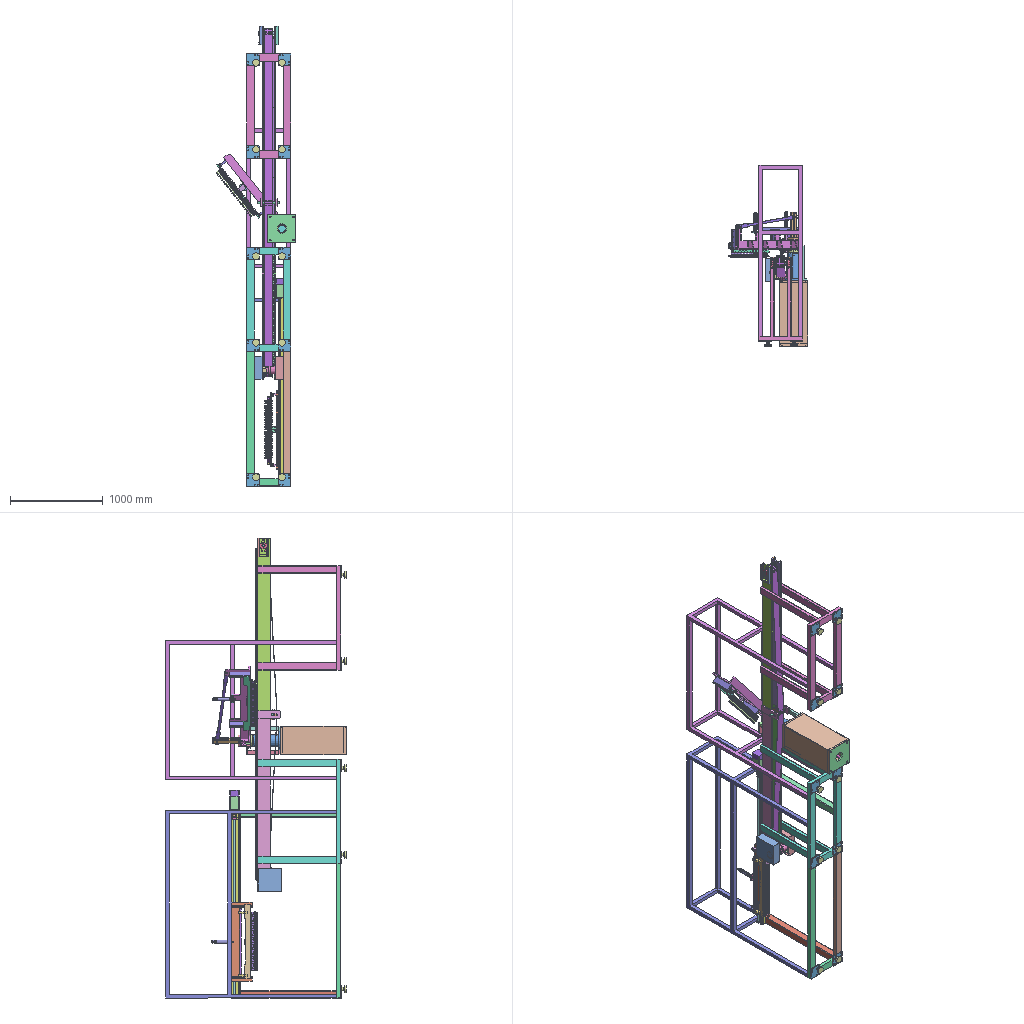Assembly | STEP file | 79 different items | 846 placed | box 859 x 1942 x 4946 mm
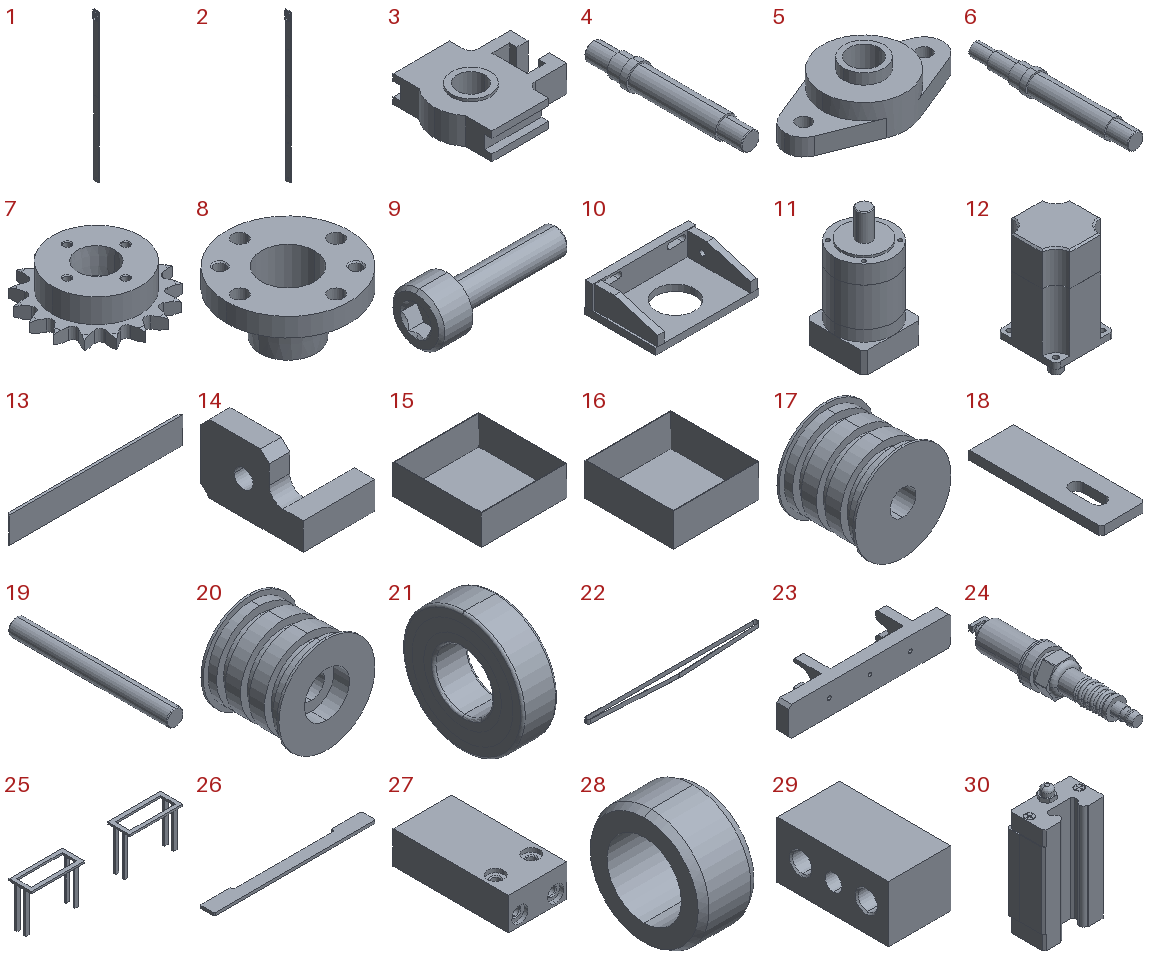Parts list (item | name | quantity | parent item | size | volume):
1 | 012-6-07-01-2 | x1 | in 12-06-07-00-2 | 51 x 134.1 x 3800 mm | 8306378 mm3
2 | 012-6-07-02-2 | x1 | in 12-06-07-00-2 | 51 x 134.1 x 3800 mm | 8297269 mm3
3 | UCT205 | x2 | in 12-06-07-00-2 | 94 x 89 x 34 mm | 126176 mm3
4 | 012-6-07-04 | x1 | in 12-06-07-00-2 | 35 x 216.4 x 35 mm | 140753 mm3
5 | UCFL205 | x2 | in 12-06-07-00-2 | 130 x 68 x 35.7 mm | 116034 mm3
6 | 012-6-07-05 | x1 | in 12-06-07-00-2 | 35 x 249.4 x 35 mm | 151867 mm3
7 | LFSP40B17_20_Asp | x2 | in LFSP40B17_20_A_LFSP40B17-20-A | 75.676 x 75.353 x 22 mm | 49189 mm3
8 | LFSP35B_20_boltbushing | x2 | in LFSP40B17_20_A_LFSP40B17-20-A | 46 x 46 x 23 mm | 9749 mm3
9 | LFSP35B20boltbolt | x8 | in LFSP40B17_20_A_LFSP40B17-20-A | 27 x 10 x 10 mm | 802.883 mm3
10 | 012-6-07-07 | x1 | in 12-06-07-00-2 | 160 x 110 x 46.5 mm | 267111 mm3
11 | PL80-40 | x2 | in 12-06-07-00-2, Reducer 2012-6-19 | 80 x 80 x 162 mm | 651730 mm3
12 | 1FL40-44-0AF21-0AA0 | x2 | in 12-06-07-00-2, Reducer 2012-6-19 | 80 x 80 x 173 mm | 725829 mm3
13 | 012-6-07-08 | x3 | in 12-06-07-00-2 | 750 x 12 x 114 mm | 828876 mm3
14 | 012-6-07-010 | x1 | in 12-06-07-00-2 | 42 x 60 x 40 mm | 27374 mm3
15 | 012-6-07-011 | x1 | in 12-06-07-00-2 | 247 x 253 x 86 mm | 291638 mm3
16 | 012-6-07-012 | x1 | in 12-06-07-00-2 | 247 x 253 x 95 mm | 309494 mm3
17 | 012-6-07-016 | x2 | in 12-06-07-00-2 | 111 x 90 x 111 mm | 582989 mm3
18 | 012-6-07-017 | x2 | in 12-06-07-00-2 | 80 x 240 x 16 mm | 282946 mm3
19 | 012-6-07-018 | x1 | in 12-06-07-00-2 | 25 x 238 x 25 mm | 116752 mm3
20 | 012-6-07-015 | x1 | in 12-06-07-00-2 | 111 x 90 x 111 mm | 531982 mm3
21 | 6205ZZ_6205ZZ | x2 | in 12-06-07-00-2 | 15 x 52 x 52 mm | 22330 mm3
22 | T10 timing belt-1-2 | x1 | in 12-06-07-00-2 | 3744 x 205.239 x 85 mm | 1293096 mm3
23 | 012-6-07-03 | x143 | in 12-06-07-01 | 110 x 27 x 20 mm | 20647 mm3
24 | FR8SES | x205 | in 12-06-07-01, 2012-06-08-00-2, xuanzhuanjixs | 18.6 x 85.1 x 18.6 mm | 9845 mm3
25 | Lower frame | x1 | in 12-06-07-00-2 | 3200 x 469.62 x 888 mm | 39914761 mm3
26 | 2012-06-08-01 | x1 | in 2012-06-08-00-2 | 800 x 70 x 14 mm | 678901 mm3
27 | - | x50 | - | 18 x 35.6 x 10 mm | 6107 mm3
28 | 189652_ZBH_5 | x100 | - | 2.4 x 5 x 5 mm | 27.025 mm3
29 | - | x100 | - | 5.5 x 9.9 x 5 mm | 236.494 mm3
30 | block_SXR24 | x4 | in 2012-06-08-00-2, xuanzhuanjixs | 34 x 20 x 63 mm | 30781 mm3
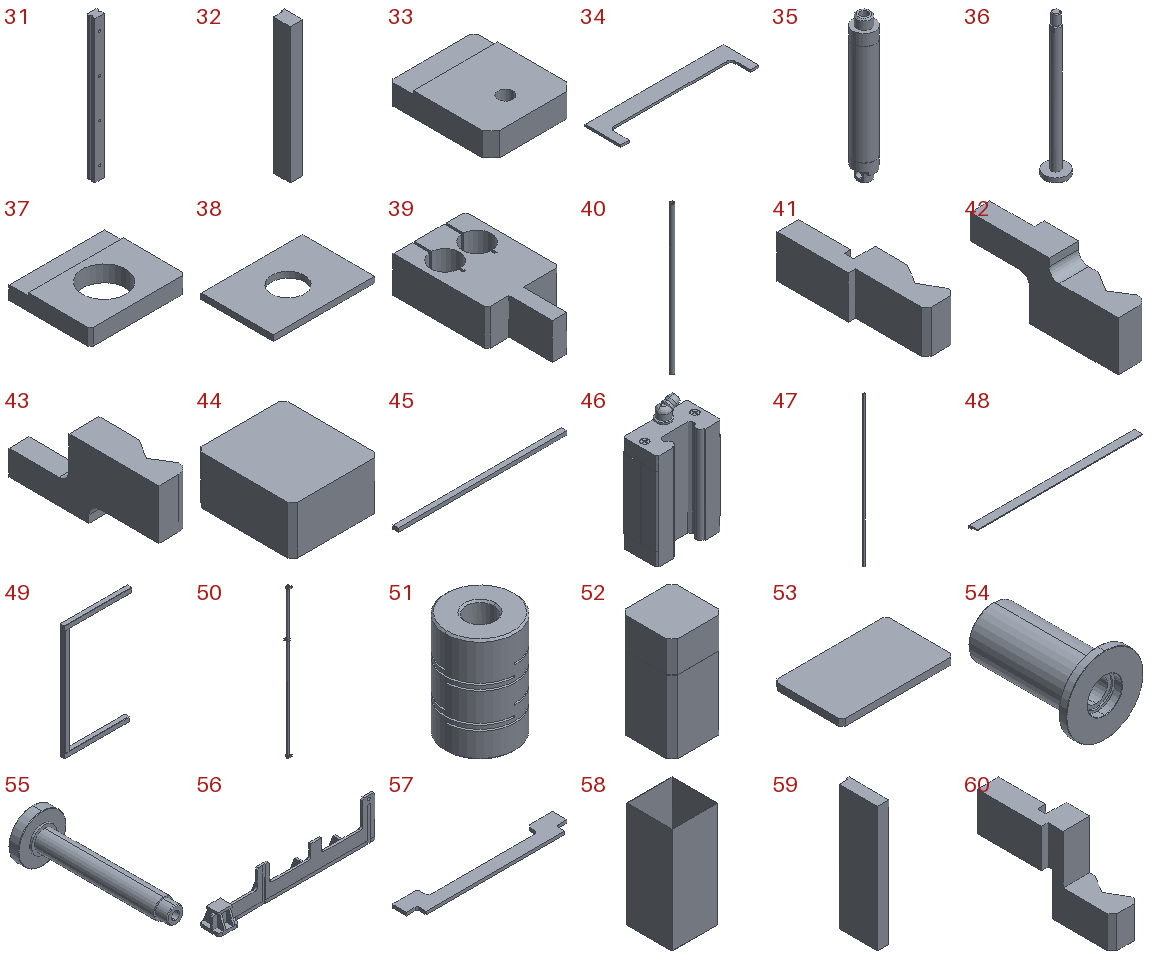31 | rail1_SXR24_220 | x4 | in 2012-06-08-00-2, xuanzhuanjixs | 15 x 12.5 x 220 mm | 36709 mm3
32 | 2012-06-08-02 | x2 | in 2012-06-08-00-2 | 20 x 30 x 220 mm | 123750 mm3
33 | 2012-06-08-03 | x1 | in 2012-06-08-00-2 | 50 x 60 x 14 mm | 39351 mm3
34 | 2012-06-08-04 | x1 | in 2012-06-08-00-2 | 850 x 220 x 14 mm | 1368448 mm3
35 | - | x2 | - | 34 x 34 x 222 mm | 66628 mm3
36 | - | x2 | - | 32 x 32 x 195.5 mm | 25619 mm3
37 | 2012-06-08-07 | x1 | in 2012-06-08-00-2 | 70 x 60 x 12 mm | 38741 mm3
38 | 2012-06-08-08 | x1 | in 2012-06-08-00-2 | 70 x 50 x 4 mm | 12410 mm3
39 | 2012-06-08-010 | x2 | in 2012-06-08-00-2 | 50 x 95 x 25 mm | 71766 mm3
40 | 2012-06-08-09 | x2 | in 2012-06-08-00-2 | 20 x 20 x 730 mm | 137949 mm3
41 | 2012-06-08-011 | x52 | in 2012-06-08-00-2, xuanzhuanjixs | 7.7 x 30 x 9 mm | 1306 mm3
42 | 2012-06-08-012 | x12 | in 2012-06-08-00-2 | 6 x 30 x 13.5 mm | 1336 mm3
43 | 2012-06-08-013 | x12 | in 2012-06-08-00-2 | 6 x 30 x 13.5 mm | 1336 mm3
44 | 2012-06-08-017 | x24 | in 2012-06-08-00-2, xuanzhuanjixs | 18 x 20 x 10 mm | 3580 mm3
45 | Cylinder hanging plate | x1 | in 2012-06-08-00-2 | 627.6 x 20 x 14 mm | 175728 mm3
46 | block_SXRB28 | x2 | in 2012-06-08-00-2 | 42 x 22 x 74.3 mm | 45231 mm3
47 | rail_SX2RZ28_280 | x1 | in 2012-06-08-00-2 | 20 x 15.5 x 2022 mm | 581693 mm3
48 | Linear bearing mounting plate | x1 | in 2012-06-08-00-2 | 2022 x 100 x 32 mm | 3400163 mm3
49 | Gantry | x1 | in 2012-06-08-00-2 | 1171 x 80 x 2022 mm | 26562153 mm3
50 | Lead screw mount | x1 | in 2012-06-08-00-2 | 60 x 50 x 1962 mm | 1004737 mm3
51 | Coupling | x1 | in 2012-06-08-00-2 | 40 x 40 x 60 mm | 58936 mm3
52 | Servo | x1 | in 2012-06-08-00-2 | 100 x 100 x 230 mm | 1946815 mm3
53 | Servo mount | x1 | in 2012-06-08-00-2 | 165 x 100 x 10 mm | 164500 mm3
54 | Backup 2012-3-22-03 | x1 | in xuanzhuanjixs | 200 x 290 x 200 mm | 3240505 mm3
55 | Backup 2012-3-22-04 | x1 | in xuanzhuanjixs | 120 x 360 x 120 mm | 913608 mm3
56 | Backup 2012-3-22-07 | x1 | in xuanzhuanjixs | 1050 x 130.1 x 270 mm | 3935848 mm3
57 | Backup 2012-3-22-09 | x1 | in xuanzhuanjixs | 730 x 105 x 14 mm | 668354 mm3
58 | Backup 2012-3-22-011 | x1 | in xuanzhuanjixs | 304 x 304 x 708.25 mm | 1711132 mm3
59 | Backup 2012-3-22-015 | x2 | in xuanzhuanjixs | 20 x 70 x 220 mm | 299750 mm3
60 | 2012-06-08-016 | x12 | in xuanzhuanjixs | 7.7 x 30 x 19 mm | 1396 mm3
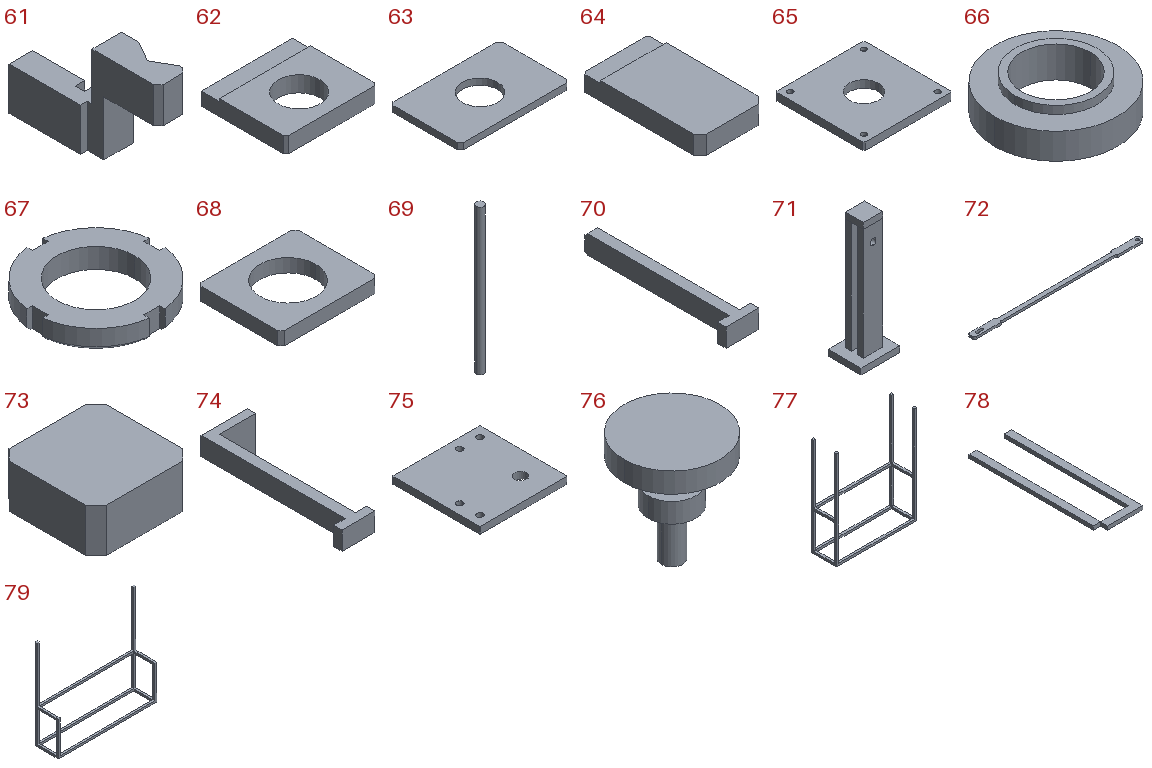61 | Mirror 2012-06-08-016 | x12 | in xuanzhuanjixs | 7.7 x 30 x 19 mm | 1396 mm3
62 | Backup 2012-3-22-012 | x1 | in xuanzhuanjixs | 70 x 65 x 12 mm | 42941 mm3
63 | Backup 2012-3-22-013 | x1 | in xuanzhuanjixs | 70 x 45 x 4 mm | 10978 mm3
64 | Backup 2012-3-22-014 | x1 | in xuanzhuanjixs | 50 x 90 x 14 mm | 61202 mm3
65 | Backup 2012-3-22-016 | x2 | in xuanzhuanjixs | 300 x 300 x 25 mm | 2035882 mm3
66 | 32210 | x2 | in xuanzhuanjixs | 90 x 90 x 24.75 mm | 82408 mm3
67 | M42 nut | x2 | in xuanzhuanjixs | 61.482 x 61.482 x 10 mm | 16995 mm3
68 | Backup 2012-3-22-017 | x1 | in xuanzhuanjixs | 140 x 120 x 19 mm | 222746 mm3
69 | Backup 2012-3-22-018 | x4 | in xuanzhuanjixs | 35 x 35 x 658.25 mm | 633311 mm3
70 | 2012-06-08-018 | x1 | in xuanzhuanjixs | 80 x 370 x 45 mm | 465125 mm3
71 | Backup 2012-3-22-019 | x1 | in xuanzhuanjixs | 90 x 76 x 288 mm | 445485 mm3
72 | Backup 2012-3-22-020 | x1 | in xuanzhuanjixs | 1020 x 40 x 14 mm | 410338 mm3
73 | 2012-06-08-019 | x2 | in xuanzhuanjixs | 45 x 45 x 20 mm | 39500 mm3
74 | Stopper | x1 | in xuanzhuanjixs | 140 x 370 x 109 mm | 624600 mm3
75 | Foot plate | x10 | in 12-06-07-00-2 | 130 x 130 x 10 mm | 164030 mm3
76 | M16 foot | x10 | in 12-06-07-00-2 | 73.343 x 73.343 x 84.032 mm | 107623 mm3
77 | Upper frame | x1 | in 12-06-07-00-2 | 1500 x 470 x 1840 mm | 21088000 mm3
78 | Connecting profile | x1 | in 12-06-07-00-2 | 469.62 x 1446 x 40.945 mm | 10095669 mm3
79 | Upper frame 2 | x1 | in 12-06-07-00-2 | 2022 x 470 x 1840 mm | 19970720 mm3
Placements (level | parent | child | x y z in mm | rotation matrix by rows), first 348 of 1046 lines:
1 | 12-06-07-00-2 | 012-6-07-01-2 | 30.237 5.383 -1250.0 | 1 0 0 0 1 0 0 0 1
1 | 12-06-07-00-2 | 012-6-07-02-2 | 160.237 5.383 -1250.0 | -1 0 0 0 -1 0 0 0 1
1 | 12-06-07-00-2 | UCT205 | -5.263 5.183 2470.5 | 0 0 1 0 1 0 -1 0 -0
1 | 12-06-07-00-2 | UCT205 | 195.737 5.183 2470.5 | 0 0 -1 0 -1 0 -1 0 0
1 | 12-06-07-00-2 | 012-6-07-04 | 203.437 5.183 2470.5 | 0 -1 0 0.9999 0 -0.01397 0.01397 0 0.9999
1 | 12-06-07-00-2 | UCFL205 | 22.237 5.383 -1170.009 | 0 0 -1 0 1 0 1 0 0
1 | 12-06-07-00-2 | UCFL205 | 168.237 5.383 -1170.009 | 0 0 1 0 -1 0 1 0 -0
1 | 12-06-07-00-2 | 012-6-07-05 | -13.463 5.383 -1170.009 | 0 1 0 -1 0 0 0 0 1
1 | 12-06-07-00-2 | LFSP40B17_20_A_LFSP40B17-20-A | 205.937 5.383 -1170.009 | 0 0 -1 0 1 0 1 0 0
2 | LFSP40B17_20_A_LFSP40B17-20-A | LFSP40B17_20_Asp | -0.0 -0.0 -0.0 | -1 0 0 0 1 0 0 0 -1
2 | LFSP40B17_20_A_LFSP40B17-20-A | LFSP35B_20_boltbushing | 0.0 0.0 -30.0 | -1 0 0 0 1 0 0 0 -1
2 | LFSP40B17_20_A_LFSP40B17-20-A | LFSP35B20boltbolt | -0.0 18.0 -36.0 | 0 0 1 0 -1 0 1 0 0
2 | LFSP40B17_20_A_LFSP40B17-20-A | LFSP35B20boltbolt | 18.0 -0.0 -36.0 | 0 0 1 0 -1 0 1 0 0
2 | LFSP40B17_20_A_LFSP40B17-20-A | LFSP35B20boltbolt | -0.0 -18.0 -36.0 | 0 0 1 0 -1 0 1 0 0
2 | LFSP40B17_20_A_LFSP40B17-20-A | LFSP35B20boltbolt | -18.0 -0.0 -36.0 | 0 0 1 0 -1 0 1 0 0
1 | 12-06-07-00-2 | 012-6-07-07 | 198.737 -125.017 -1150.1 | 0 0 -1 0 1 0 1 0 0
1 | 12-06-07-00-2 | PL80-40 | 66.737 -130.117 -1150.1 | 0 0 1 0 1 0 -1 0 -0
1 | 12-06-07-00-2 | LFSP40B17_20_A_LFSP40B17-20-A | 205.937 -130.117 -1150.1 | 0 0 -1 0 1 0 1 0 0
2 | LFSP40B17_20_A_LFSP40B17-20-A | LFSP40B17_20_Asp | -0.0 -0.0 -0.0 | -1 0 0 0 1 0 0 0 -1
2 | LFSP40B17_20_A_LFSP40B17-20-A | LFSP35B_20_boltbushing | 0.0 0.0 -30.0 | -1 0 0 0 1 0 0 0 -1
2 | LFSP40B17_20_A_LFSP40B17-20-A | LFSP35B20boltbolt | -0.0 18.0 -36.0 | 0 0 1 0 -1 0 1 0 0
2 | LFSP40B17_20_A_LFSP40B17-20-A | LFSP35B20boltbolt | 18.0 -0.0 -36.0 | 0 0 1 0 -1 0 1 0 0
2 | LFSP40B17_20_A_LFSP40B17-20-A | LFSP35B20boltbolt | -0.0 -18.0 -36.0 | 0 0 1 0 -1 0 1 0 0
2 | LFSP40B17_20_A_LFSP40B17-20-A | LFSP35B20boltbolt | -18.0 -0.0 -36.0 | 0 0 1 0 -1 0 1 0 0
1 | 12-06-07-00-2 | 1FL40-44-0AF21-0AA0 | 66.737 -130.117 -1150.1 | 0 0 -1 0 1 0 1 0 0
1 | 12-06-07-00-2 | 012-6-07-08 | 38.237 49.183 2045.0 | 0 0 1 0 1 0 -1 0 -0
1 | 12-06-07-00-2 | 012-6-07-08 | 38.237 49.183 545.0 | 0 0 1 0 1 0 -1 0 -0
1 | 12-06-07-00-2 | 012-6-07-08 | 38.237 49.183 1295.0 | 0 0 1 0 1 0 -1 0 -0
1 | 12-06-07-00-2 | 012-6-07-010 | 152.237 -70.117 -1033.1 | 0 0 1 0 -1 0 1 0 -0
1 | 12-06-07-00-2 | 012-6-07-011 | 254.237 -62.517 -1126.5 | 0 0 -1 0 1 0 1 0 0
1 | 12-06-07-00-2 | 012-6-07-012 | -72.763 -62.517 -1126.5 | 0 0 1 0 1 0 -1 0 0
1 | 12-06-07-00-2 | 012-6-07-016 | 150.237 5.183 2470.5 | 0 -1 0 1 0 0 0 0 1
1 | 12-06-07-00-2 | 012-6-07-016 | 40.237 5.383 -1170.009 | 0 1 0 -1 0 0 0 0 1
1 | 12-06-07-00-2 | 012-6-07-017 | 6.237 -56.017 650.05 | 0 0 1 0 1 0 -1 0 0
1 | 12-06-07-00-2 | 012-6-07-017 | 184.237 -56.017 650.05 | 0 0 -1 0 1 0 1 0 -0
1 | 12-06-07-00-2 | 012-6-07-018 | 214.237 -91.017 650.05 | 0 -1 0 1 0 0 0 0 1
1 | 12-06-07-00-2 | 012-6-07-015 | 25.237 -91.017 650.05 | 0 1 0 -1 0 0 0 0 1
1 | 12-06-07-00-2 | 6205ZZ_6205ZZ | 129.737 -91.017 650.05 | 1 0 0 0 1 0 0 0 1
1 | 12-06-07-00-2 | 6205ZZ_6205ZZ | 60.737 -91.017 650.05 | -1 0 0 0 -0.3818 0.9242 0 0.9242 0.3818
1 | 12-06-07-00-2 | T10 timing belt-1-2 | 137.737 5.382 -1170.005 | 0 0 -1 0.003284 1 0 1 -0.003284 0
1 | 12-06-07-00-2 | 12-06-07-01 | 102.7 67.54 2420.0 | 1 0 0 0 1 0 0 0 1
2 | 12-06-07-01 | 012-6-07-03 | -26.463 -2.157 -0.0 | 1 0 0 0 1 0 0 0 1
2 | 12-06-07-01 | FR8SES | 34.437 11.843 10.0 | 0 -1 0 0.3058 0 0.9521 -0.9521 0 0.3058
1 | 12-06-07-00-2 | 12-06-07-01 | 102.7 67.54 2395.0 | 1 0 0 0 1 0 0 0 1
2 | 12-06-07-01 | 012-6-07-03 | -26.463 -2.157 -0.0 | 1 0 0 0 1 0 0 0 1
2 | 12-06-07-01 | FR8SES | 34.437 11.843 10.0 | 0 -1 0 0.3058 0 0.9521 -0.9521 0 0.3058
1 | 12-06-07-00-2 | 12-06-07-01 | 102.7 67.54 2370.0 | 1 0 0 0 1 0 0 0 1
2 | 12-06-07-01 | 012-6-07-03 | -26.463 -2.157 -0.0 | 1 0 0 0 1 0 0 0 1
2 | 12-06-07-01 | FR8SES | 34.437 11.843 10.0 | 0 -1 0 0.3058 0 0.9521 -0.9521 0 0.3058
1 | 12-06-07-00-2 | 12-06-07-01 | 102.7 67.54 2345.0 | 1 0 0 0 1 0 0 0 1
2 | 12-06-07-01 | 012-6-07-03 | -26.463 -2.157 -0.0 | 1 0 0 0 1 0 0 0 1
2 | 12-06-07-01 | FR8SES | 34.437 11.843 10.0 | 0 -1 0 0.3058 0 0.9521 -0.9521 0 0.3058
1 | 12-06-07-00-2 | 12-06-07-01 | 102.7 67.54 2320.0 | 1 0 0 0 1 0 0 0 1
2 | 12-06-07-01 | 012-6-07-03 | -26.463 -2.157 -0.0 | 1 0 0 0 1 0 0 0 1
2 | 12-06-07-01 | FR8SES | 34.437 11.843 10.0 | 0 -1 0 0.3058 0 0.9521 -0.9521 0 0.3058
1 | 12-06-07-00-2 | 12-06-07-01 | 102.7 67.54 2295.0 | 1 0 0 0 1 0 0 0 1
2 | 12-06-07-01 | 012-6-07-03 | -26.463 -2.157 -0.0 | 1 0 0 0 1 0 0 0 1
2 | 12-06-07-01 | FR8SES | 34.437 11.843 10.0 | 0 -1 0 0.3058 0 0.9521 -0.9521 0 0.3058
1 | 12-06-07-00-2 | 12-06-07-01 | 102.7 67.54 2270.0 | 1 0 0 0 1 0 0 0 1
2 | 12-06-07-01 | 012-6-07-03 | -26.463 -2.157 -0.0 | 1 0 0 0 1 0 0 0 1
2 | 12-06-07-01 | FR8SES | 34.437 11.843 10.0 | 0 -1 0 0.3058 0 0.9521 -0.9521 0 0.3058
1 | 12-06-07-00-2 | 12-06-07-01 | 102.7 67.54 2245.0 | 1 0 0 0 1 0 0 0 1
2 | 12-06-07-01 | 012-6-07-03 | -26.463 -2.157 -0.0 | 1 0 0 0 1 0 0 0 1
2 | 12-06-07-01 | FR8SES | 34.437 11.843 10.0 | 0 -1 0 0.3058 0 0.9521 -0.9521 0 0.3058
1 | 12-06-07-00-2 | 12-06-07-01 | 102.7 67.54 2220.0 | 1 0 0 0 1 0 0 0 1
2 | 12-06-07-01 | 012-6-07-03 | -26.463 -2.157 -0.0 | 1 0 0 0 1 0 0 0 1
2 | 12-06-07-01 | FR8SES | 34.437 11.843 10.0 | 0 -1 0 0.3058 0 0.9521 -0.9521 0 0.3058
1 | 12-06-07-00-2 | 12-06-07-01 | 102.7 67.54 2195.0 | 1 0 0 0 1 0 0 0 1
2 | 12-06-07-01 | 012-6-07-03 | -26.463 -2.157 -0.0 | 1 0 0 0 1 0 0 0 1
2 | 12-06-07-01 | FR8SES | 34.437 11.843 10.0 | 0 -1 0 0.3058 0 0.9521 -0.9521 0 0.3058
1 | 12-06-07-00-2 | 12-06-07-01 | 102.7 67.54 2170.0 | 1 0 0 0 1 0 0 0 1
2 | 12-06-07-01 | 012-6-07-03 | -26.463 -2.157 -0.0 | 1 0 0 0 1 0 0 0 1
2 | 12-06-07-01 | FR8SES | 34.437 11.843 10.0 | 0 -1 0 0.3058 0 0.9521 -0.9521 0 0.3058
1 | 12-06-07-00-2 | 12-06-07-01 | 102.7 67.54 2145.0 | 1 0 0 0 1 0 0 0 1
2 | 12-06-07-01 | 012-6-07-03 | -26.463 -2.157 -0.0 | 1 0 0 0 1 0 0 0 1
2 | 12-06-07-01 | FR8SES | 34.437 11.843 10.0 | 0 -1 0 0.3058 0 0.9521 -0.9521 0 0.3058
1 | 12-06-07-00-2 | 12-06-07-01 | 102.7 67.54 2120.0 | 1 0 0 0 1 0 0 0 1
2 | 12-06-07-01 | 012-6-07-03 | -26.463 -2.157 -0.0 | 1 0 0 0 1 0 0 0 1
2 | 12-06-07-01 | FR8SES | 34.437 11.843 10.0 | 0 -1 0 0.3058 0 0.9521 -0.9521 0 0.3058
1 | 12-06-07-00-2 | 12-06-07-01 | 102.7 67.54 2095.0 | 1 0 0 0 1 0 0 0 1
2 | 12-06-07-01 | 012-6-07-03 | -26.463 -2.157 -0.0 | 1 0 0 0 1 0 0 0 1
2 | 12-06-07-01 | FR8SES | 34.437 11.843 10.0 | 0 -1 0 0.3058 0 0.9521 -0.9521 0 0.3058
1 | 12-06-07-00-2 | 12-06-07-01 | 102.7 67.54 2070.0 | 1 0 0 0 1 0 0 0 1
2 | 12-06-07-01 | 012-6-07-03 | -26.463 -2.157 -0.0 | 1 0 0 0 1 0 0 0 1
2 | 12-06-07-01 | FR8SES | 34.437 11.843 10.0 | 0 -1 0 0.3058 0 0.9521 -0.9521 0 0.3058
1 | 12-06-07-00-2 | 12-06-07-01 | 102.7 67.54 2045.0 | 1 0 0 0 1 0 0 0 1
2 | 12-06-07-01 | 012-6-07-03 | -26.463 -2.157 -0.0 | 1 0 0 0 1 0 0 0 1
2 | 12-06-07-01 | FR8SES | 34.437 11.843 10.0 | 0 -1 0 0.3058 0 0.9521 -0.9521 0 0.3058
1 | 12-06-07-00-2 | 12-06-07-01 | 102.7 67.54 2020.0 | 1 0 0 0 1 0 0 0 1
2 | 12-06-07-01 | 012-6-07-03 | -26.463 -2.157 -0.0 | 1 0 0 0 1 0 0 0 1
2 | 12-06-07-01 | FR8SES | 34.437 11.843 10.0 | 0 -1 0 0.3058 0 0.9521 -0.9521 0 0.3058
1 | 12-06-07-00-2 | 12-06-07-01 | 102.7 67.54 1995.0 | 1 0 0 0 1 0 0 0 1
2 | 12-06-07-01 | 012-6-07-03 | -26.463 -2.157 -0.0 | 1 0 0 0 1 0 0 0 1
2 | 12-06-07-01 | FR8SES | 34.437 11.843 10.0 | 0 -1 0 0.3058 0 0.9521 -0.9521 0 0.3058
1 | 12-06-07-00-2 | 12-06-07-01 | 102.7 67.54 1970.0 | 1 0 0 0 1 0 0 0 1
2 | 12-06-07-01 | 012-6-07-03 | -26.463 -2.157 -0.0 | 1 0 0 0 1 0 0 0 1
2 | 12-06-07-01 | FR8SES | 34.437 11.843 10.0 | 0 -1 0 0.3058 0 0.9521 -0.9521 0 0.3058
1 | 12-06-07-00-2 | 12-06-07-01 | 102.7 67.54 1945.0 | 1 0 0 0 1 0 0 0 1
2 | 12-06-07-01 | 012-6-07-03 | -26.463 -2.157 -0.0 | 1 0 0 0 1 0 0 0 1
2 | 12-06-07-01 | FR8SES | 34.437 11.843 10.0 | 0 -1 0 0.3058 0 0.9521 -0.9521 0 0.3058
1 | 12-06-07-00-2 | 12-06-07-01 | 102.7 67.54 1920.0 | 1 0 0 0 1 0 0 0 1
2 | 12-06-07-01 | 012-6-07-03 | -26.463 -2.157 -0.0 | 1 0 0 0 1 0 0 0 1
2 | 12-06-07-01 | FR8SES | 34.437 11.843 10.0 | 0 -1 0 0.3058 0 0.9521 -0.9521 0 0.3058
1 | 12-06-07-00-2 | 12-06-07-01 | 102.7 67.54 1895.0 | 1 0 0 0 1 0 0 0 1
2 | 12-06-07-01 | 012-6-07-03 | -26.463 -2.157 -0.0 | 1 0 0 0 1 0 0 0 1
2 | 12-06-07-01 | FR8SES | 34.437 11.843 10.0 | 0 -1 0 0.3058 0 0.9521 -0.9521 0 0.3058
1 | 12-06-07-00-2 | 12-06-07-01 | 102.7 67.54 1870.0 | 1 0 0 0 1 0 0 0 1
2 | 12-06-07-01 | 012-6-07-03 | -26.463 -2.157 -0.0 | 1 0 0 0 1 0 0 0 1
2 | 12-06-07-01 | FR8SES | 34.437 11.843 10.0 | 0 -1 0 0.3058 0 0.9521 -0.9521 0 0.3058
1 | 12-06-07-00-2 | 12-06-07-01 | 102.7 67.54 1845.0 | 1 0 0 0 1 0 0 0 1
2 | 12-06-07-01 | 012-6-07-03 | -26.463 -2.157 -0.0 | 1 0 0 0 1 0 0 0 1
2 | 12-06-07-01 | FR8SES | 34.437 11.843 10.0 | 0 -1 0 0.3058 0 0.9521 -0.9521 0 0.3058
1 | 12-06-07-00-2 | 12-06-07-01 | 102.7 67.54 1820.0 | 1 0 0 0 1 0 0 0 1
2 | 12-06-07-01 | 012-6-07-03 | -26.463 -2.157 -0.0 | 1 0 0 0 1 0 0 0 1
2 | 12-06-07-01 | FR8SES | 34.437 11.843 10.0 | 0 -1 0 0.3058 0 0.9521 -0.9521 0 0.3058
1 | 12-06-07-00-2 | 12-06-07-01 | 102.7 67.54 1795.0 | 1 0 0 0 1 0 0 0 1
2 | 12-06-07-01 | 012-6-07-03 | -26.463 -2.157 -0.0 | 1 0 0 0 1 0 0 0 1
2 | 12-06-07-01 | FR8SES | 34.437 11.843 10.0 | 0 -1 0 0.3058 0 0.9521 -0.9521 0 0.3058
1 | 12-06-07-00-2 | 12-06-07-01 | 102.7 67.54 1770.0 | 1 0 0 0 1 0 0 0 1
2 | 12-06-07-01 | 012-6-07-03 | -26.463 -2.157 -0.0 | 1 0 0 0 1 0 0 0 1
2 | 12-06-07-01 | FR8SES | 34.437 11.843 10.0 | 0 -1 0 0.3058 0 0.9521 -0.9521 0 0.3058
1 | 12-06-07-00-2 | 12-06-07-01 | 102.7 67.54 1745.0 | 1 0 0 0 1 0 0 0 1
2 | 12-06-07-01 | 012-6-07-03 | -26.463 -2.157 -0.0 | 1 0 0 0 1 0 0 0 1
2 | 12-06-07-01 | FR8SES | 34.437 11.843 10.0 | 0 -1 0 0.3058 0 0.9521 -0.9521 0 0.3058
1 | 12-06-07-00-2 | 12-06-07-01 | 102.7 67.54 1720.0 | 1 0 0 0 1 0 0 0 1
2 | 12-06-07-01 | 012-6-07-03 | -26.463 -2.157 -0.0 | 1 0 0 0 1 0 0 0 1
2 | 12-06-07-01 | FR8SES | 34.437 11.843 10.0 | 0 -1 0 0.3058 0 0.9521 -0.9521 0 0.3058
1 | 12-06-07-00-2 | 12-06-07-01 | 102.7 67.54 1695.0 | 1 0 0 0 1 0 0 0 1
2 | 12-06-07-01 | 012-6-07-03 | -26.463 -2.157 -0.0 | 1 0 0 0 1 0 0 0 1
2 | 12-06-07-01 | FR8SES | 34.437 11.843 10.0 | 0 -1 0 0.3058 0 0.9521 -0.9521 0 0.3058
1 | 12-06-07-00-2 | 12-06-07-01 | 102.7 67.54 1670.0 | 1 0 0 0 1 0 0 0 1
2 | 12-06-07-01 | 012-6-07-03 | -26.463 -2.157 -0.0 | 1 0 0 0 1 0 0 0 1
2 | 12-06-07-01 | FR8SES | 34.437 11.843 10.0 | 0 -1 0 0.3058 0 0.9521 -0.9521 0 0.3058
1 | 12-06-07-00-2 | 12-06-07-01 | 102.7 67.54 1645.0 | 1 0 0 0 1 0 0 0 1
2 | 12-06-07-01 | 012-6-07-03 | -26.463 -2.157 -0.0 | 1 0 0 0 1 0 0 0 1
2 | 12-06-07-01 | FR8SES | 34.437 11.843 10.0 | 0 -1 0 0.3058 0 0.9521 -0.9521 0 0.3058
1 | 12-06-07-00-2 | 12-06-07-01 | 102.7 67.54 1620.0 | 1 0 0 0 1 0 0 0 1
2 | 12-06-07-01 | 012-6-07-03 | -26.463 -2.157 -0.0 | 1 0 0 0 1 0 0 0 1
2 | 12-06-07-01 | FR8SES | 34.437 11.843 10.0 | 0 -1 0 0.3058 0 0.9521 -0.9521 0 0.3058
1 | 12-06-07-00-2 | 12-06-07-01 | 102.7 67.54 1595.0 | 1 0 0 0 1 0 0 0 1
2 | 12-06-07-01 | 012-6-07-03 | -26.463 -2.157 -0.0 | 1 0 0 0 1 0 0 0 1
2 | 12-06-07-01 | FR8SES | 34.437 11.843 10.0 | 0 -1 0 0.3058 0 0.9521 -0.9521 0 0.3058
1 | 12-06-07-00-2 | 12-06-07-01 | 102.7 67.54 1570.0 | 1 0 0 0 1 0 0 0 1
2 | 12-06-07-01 | 012-6-07-03 | -26.463 -2.157 -0.0 | 1 0 0 0 1 0 0 0 1
2 | 12-06-07-01 | FR8SES | 34.437 11.843 10.0 | 0 -1 0 0.3058 0 0.9521 -0.9521 0 0.3058
1 | 12-06-07-00-2 | 12-06-07-01 | 102.7 67.54 1545.0 | 1 0 0 0 1 0 0 0 1
2 | 12-06-07-01 | 012-6-07-03 | -26.463 -2.157 -0.0 | 1 0 0 0 1 0 0 0 1
2 | 12-06-07-01 | FR8SES | 34.437 11.843 10.0 | 0 -1 0 0.3058 0 0.9521 -0.9521 0 0.3058
1 | 12-06-07-00-2 | 12-06-07-01 | 102.7 67.54 1520.0 | 1 0 0 0 1 0 0 0 1
2 | 12-06-07-01 | 012-6-07-03 | -26.463 -2.157 -0.0 | 1 0 0 0 1 0 0 0 1
2 | 12-06-07-01 | FR8SES | 34.437 11.843 10.0 | 0 -1 0 0.3058 0 0.9521 -0.9521 0 0.3058
1 | 12-06-07-00-2 | 12-06-07-01 | 102.7 67.54 1495.0 | 1 0 0 0 1 0 0 0 1
2 | 12-06-07-01 | 012-6-07-03 | -26.463 -2.157 -0.0 | 1 0 0 0 1 0 0 0 1
2 | 12-06-07-01 | FR8SES | 34.437 11.843 10.0 | 0 -1 0 0.3058 0 0.9521 -0.9521 0 0.3058
1 | 12-06-07-00-2 | 12-06-07-01 | 102.7 67.54 1470.0 | 1 0 0 0 1 0 0 0 1
2 | 12-06-07-01 | 012-6-07-03 | -26.463 -2.157 -0.0 | 1 0 0 0 1 0 0 0 1
2 | 12-06-07-01 | FR8SES | 34.437 11.843 10.0 | 0 -1 0 0.3058 0 0.9521 -0.9521 0 0.3058
1 | 12-06-07-00-2 | 12-06-07-01 | 102.7 67.54 1445.0 | 1 0 0 0 1 0 0 0 1
2 | 12-06-07-01 | 012-6-07-03 | -26.463 -2.157 -0.0 | 1 0 0 0 1 0 0 0 1
2 | 12-06-07-01 | FR8SES | 34.437 11.843 10.0 | 0 -1 0 0.3058 0 0.9521 -0.9521 0 0.3058
1 | 12-06-07-00-2 | 12-06-07-01 | 102.7 67.54 1420.0 | 1 0 0 0 1 0 0 0 1
2 | 12-06-07-01 | 012-6-07-03 | -26.463 -2.157 -0.0 | 1 0 0 0 1 0 0 0 1
2 | 12-06-07-01 | FR8SES | 34.437 11.843 10.0 | 0 -1 0 0.3058 0 0.9521 -0.9521 0 0.3058
1 | 12-06-07-00-2 | 12-06-07-01 | 102.7 67.54 1395.0 | 1 0 0 0 1 0 0 0 1
2 | 12-06-07-01 | 012-6-07-03 | -26.463 -2.157 -0.0 | 1 0 0 0 1 0 0 0 1
2 | 12-06-07-01 | FR8SES | 34.437 11.843 10.0 | 0 -1 0 0.3058 0 0.9521 -0.9521 0 0.3058
1 | 12-06-07-00-2 | 12-06-07-01 | 102.7 67.54 1370.0 | 1 0 0 0 1 0 0 0 1
2 | 12-06-07-01 | 012-6-07-03 | -26.463 -2.157 -0.0 | 1 0 0 0 1 0 0 0 1
2 | 12-06-07-01 | FR8SES | 34.437 11.843 10.0 | 0 -1 0 0.3058 0 0.9521 -0.9521 0 0.3058
1 | 12-06-07-00-2 | 12-06-07-01 | 102.7 67.54 1345.0 | 1 0 0 0 1 0 0 0 1
2 | 12-06-07-01 | 012-6-07-03 | -26.463 -2.157 -0.0 | 1 0 0 0 1 0 0 0 1
2 | 12-06-07-01 | FR8SES | 34.437 11.843 10.0 | 0 -1 0 0.3058 0 0.9521 -0.9521 0 0.3058
1 | 12-06-07-00-2 | 12-06-07-01 | 102.7 67.54 1320.0 | 1 0 0 0 1 0 0 0 1
2 | 12-06-07-01 | 012-6-07-03 | -26.463 -2.157 -0.0 | 1 0 0 0 1 0 0 0 1
2 | 12-06-07-01 | FR8SES | 34.437 11.843 10.0 | 0 -1 0 0.3058 0 0.9521 -0.9521 0 0.3058
1 | 12-06-07-00-2 | 12-06-07-01 | 102.7 67.54 1295.0 | 1 0 0 0 1 0 0 0 1
2 | 12-06-07-01 | 012-6-07-03 | -26.463 -2.157 -0.0 | 1 0 0 0 1 0 0 0 1
2 | 12-06-07-01 | FR8SES | 34.437 11.843 10.0 | 0 -1 0 0.3058 0 0.9521 -0.9521 0 0.3058
1 | 12-06-07-00-2 | 12-06-07-01 | 102.7 67.54 1270.0 | 1 0 0 0 1 0 0 0 1
2 | 12-06-07-01 | 012-6-07-03 | -26.463 -2.157 -0.0 | 1 0 0 0 1 0 0 0 1
2 | 12-06-07-01 | FR8SES | 34.437 11.843 10.0 | 0 -1 0 0.3058 0 0.9521 -0.9521 0 0.3058
1 | 12-06-07-00-2 | 12-06-07-01 | 102.7 67.54 1245.0 | 1 0 0 0 1 0 0 0 1
2 | 12-06-07-01 | 012-6-07-03 | -26.463 -2.157 -0.0 | 1 0 0 0 1 0 0 0 1
2 | 12-06-07-01 | FR8SES | 34.437 11.843 10.0 | 0 -1 0 0.3058 0 0.9521 -0.9521 0 0.3058
1 | 12-06-07-00-2 | 12-06-07-01 | 102.7 67.54 1220.0 | 1 0 0 0 1 0 0 0 1
2 | 12-06-07-01 | 012-6-07-03 | -26.463 -2.157 -0.0 | 1 0 0 0 1 0 0 0 1
2 | 12-06-07-01 | FR8SES | 34.437 11.843 10.0 | 0 -1 0 0.3058 0 0.9521 -0.9521 0 0.3058
1 | 12-06-07-00-2 | 12-06-07-01 | 102.7 67.54 1195.0 | 1 0 0 0 1 0 0 0 1
2 | 12-06-07-01 | 012-6-07-03 | -26.463 -2.157 -0.0 | 1 0 0 0 1 0 0 0 1
2 | 12-06-07-01 | FR8SES | 34.437 11.843 10.0 | 0 -1 0 0.3058 0 0.9521 -0.9521 0 0.3058
1 | 12-06-07-00-2 | 12-06-07-01 | 102.7 67.54 1170.0 | 1 0 0 0 1 0 0 0 1
2 | 12-06-07-01 | 012-6-07-03 | -26.463 -2.157 -0.0 | 1 0 0 0 1 0 0 0 1
2 | 12-06-07-01 | FR8SES | 34.437 11.843 10.0 | 0 -1 0 0.3058 0 0.9521 -0.9521 0 0.3058
1 | 12-06-07-00-2 | 12-06-07-01 | 102.7 67.54 1145.0 | 1 0 0 0 1 0 0 0 1
2 | 12-06-07-01 | 012-6-07-03 | -26.463 -2.157 -0.0 | 1 0 0 0 1 0 0 0 1
2 | 12-06-07-01 | FR8SES | 34.437 11.843 10.0 | 0 -1 0 0.3058 0 0.9521 -0.9521 0 0.3058
1 | 12-06-07-00-2 | 12-06-07-01 | 102.7 67.54 1120.0 | 1 0 0 0 1 0 0 0 1
2 | 12-06-07-01 | 012-6-07-03 | -26.463 -2.157 -0.0 | 1 0 0 0 1 0 0 0 1
2 | 12-06-07-01 | FR8SES | 34.437 11.843 10.0 | 0 -1 0 0.3058 0 0.9521 -0.9521 0 0.3058
1 | 12-06-07-00-2 | 12-06-07-01 | 102.7 67.54 1095.0 | 1 0 0 0 1 0 0 0 1
2 | 12-06-07-01 | 012-6-07-03 | -26.463 -2.157 -0.0 | 1 0 0 0 1 0 0 0 1
2 | 12-06-07-01 | FR8SES | 34.437 11.843 10.0 | 0 -1 0 0.3058 0 0.9521 -0.9521 0 0.3058
1 | 12-06-07-00-2 | 12-06-07-01 | 102.7 67.54 1070.0 | 1 0 0 0 1 0 0 0 1
2 | 12-06-07-01 | 012-6-07-03 | -26.463 -2.157 -0.0 | 1 0 0 0 1 0 0 0 1
2 | 12-06-07-01 | FR8SES | 34.437 11.843 10.0 | 0 -1 0 0.3058 0 0.9521 -0.9521 0 0.3058
1 | 12-06-07-00-2 | 12-06-07-01 | 102.7 67.54 1045.0 | 1 0 0 0 1 0 0 0 1
2 | 12-06-07-01 | 012-6-07-03 | -26.463 -2.157 -0.0 | 1 0 0 0 1 0 0 0 1
2 | 12-06-07-01 | FR8SES | 34.437 11.843 10.0 | 0 -1 0 0.3058 0 0.9521 -0.9521 0 0.3058
1 | 12-06-07-00-2 | 12-06-07-01 | 102.7 67.54 1020.0 | 1 0 0 0 1 0 0 0 1
2 | 12-06-07-01 | 012-6-07-03 | -26.463 -2.157 -0.0 | 1 0 0 0 1 0 0 0 1
2 | 12-06-07-01 | FR8SES | 34.437 11.843 10.0 | 0 -1 0 0.3058 0 0.9521 -0.9521 0 0.3058
1 | 12-06-07-00-2 | 12-06-07-01 | 102.7 67.54 995.0 | 1 0 0 0 1 0 0 0 1
2 | 12-06-07-01 | 012-6-07-03 | -26.463 -2.157 -0.0 | 1 0 0 0 1 0 0 0 1
2 | 12-06-07-01 | FR8SES | 34.437 11.843 10.0 | 0 -1 0 0.3058 0 0.9521 -0.9521 0 0.3058
1 | 12-06-07-00-2 | 12-06-07-01 | 102.7 67.54 970.0 | 1 0 0 0 1 0 0 0 1
2 | 12-06-07-01 | 012-6-07-03 | -26.463 -2.157 -0.0 | 1 0 0 0 1 0 0 0 1
2 | 12-06-07-01 | FR8SES | 34.437 11.843 10.0 | 0 -1 0 0.3058 0 0.9521 -0.9521 0 0.3058
1 | 12-06-07-00-2 | 12-06-07-01 | 102.7 67.54 945.0 | 1 0 0 0 1 0 0 0 1
2 | 12-06-07-01 | 012-6-07-03 | -26.463 -2.157 -0.0 | 1 0 0 0 1 0 0 0 1
2 | 12-06-07-01 | FR8SES | 34.437 11.843 10.0 | 0 -1 0 0.3058 0 0.9521 -0.9521 0 0.3058
1 | 12-06-07-00-2 | 12-06-07-01 | 102.7 67.54 920.0 | 1 0 0 0 1 0 0 0 1
2 | 12-06-07-01 | 012-6-07-03 | -26.463 -2.157 -0.0 | 1 0 0 0 1 0 0 0 1
2 | 12-06-07-01 | FR8SES | 34.437 11.843 10.0 | 0 -1 0 0.3058 0 0.9521 -0.9521 0 0.3058
1 | 12-06-07-00-2 | 12-06-07-01 | 102.7 67.54 895.0 | 1 0 0 0 1 0 0 0 1
2 | 12-06-07-01 | 012-6-07-03 | -26.463 -2.157 -0.0 | 1 0 0 0 1 0 0 0 1
2 | 12-06-07-01 | FR8SES | 34.437 11.843 10.0 | 0 -1 0 0.3058 0 0.9521 -0.9521 0 0.3058
1 | 12-06-07-00-2 | 12-06-07-01 | 102.7 67.54 870.0 | 1 0 0 0 1 0 0 0 1
2 | 12-06-07-01 | 012-6-07-03 | -26.463 -2.157 -0.0 | 1 0 0 0 1 0 0 0 1
2 | 12-06-07-01 | FR8SES | 34.437 11.843 10.0 | 0 -1 0 0.3058 0 0.9521 -0.9521 0 0.3058
1 | 12-06-07-00-2 | 12-06-07-01 | 102.7 67.54 845.0 | 1 0 0 0 1 0 0 0 1
2 | 12-06-07-01 | 012-6-07-03 | -26.463 -2.157 -0.0 | 1 0 0 0 1 0 0 0 1
2 | 12-06-07-01 | FR8SES | 34.437 11.843 10.0 | 0 -1 0 0.3058 0 0.9521 -0.9521 0 0.3058
1 | 12-06-07-00-2 | 12-06-07-01 | 102.7 67.54 820.0 | 1 0 0 0 1 0 0 0 1
2 | 12-06-07-01 | 012-6-07-03 | -26.463 -2.157 -0.0 | 1 0 0 0 1 0 0 0 1
2 | 12-06-07-01 | FR8SES | 34.437 11.843 10.0 | 0 -1 0 0.3058 0 0.9521 -0.9521 0 0.3058
1 | 12-06-07-00-2 | 12-06-07-01 | 102.7 67.54 795.0 | 1 0 0 0 1 0 0 0 1
2 | 12-06-07-01 | 012-6-07-03 | -26.463 -2.157 -0.0 | 1 0 0 0 1 0 0 0 1
2 | 12-06-07-01 | FR8SES | 34.437 11.843 10.0 | 0 -1 0 0.3058 0 0.9521 -0.9521 0 0.3058
1 | 12-06-07-00-2 | 12-06-07-01 | 102.7 67.54 770.0 | 1 0 0 0 1 0 0 0 1
2 | 12-06-07-01 | 012-6-07-03 | -26.463 -2.157 -0.0 | 1 0 0 0 1 0 0 0 1
2 | 12-06-07-01 | FR8SES | 34.437 11.843 10.0 | 0 -1 0 0.3058 0 0.9521 -0.9521 0 0.3058
1 | 12-06-07-00-2 | 12-06-07-01 | 102.7 67.54 745.0 | 1 0 0 0 1 0 0 0 1
2 | 12-06-07-01 | 012-6-07-03 | -26.463 -2.157 -0.0 | 1 0 0 0 1 0 0 0 1
2 | 12-06-07-01 | FR8SES | 34.437 11.843 10.0 | 0 -1 0 0.3058 0 0.9521 -0.9521 0 0.3058
1 | 12-06-07-00-2 | 12-06-07-01 | 102.7 67.54 720.0 | 1 0 0 0 1 0 0 0 1
2 | 12-06-07-01 | 012-6-07-03 | -26.463 -2.157 -0.0 | 1 0 0 0 1 0 0 0 1
2 | 12-06-07-01 | FR8SES | 34.437 11.843 10.0 | 0 -1 0 0.3058 0 0.9521 -0.9521 0 0.3058
1 | 12-06-07-00-2 | 12-06-07-01 | 102.7 67.54 695.0 | 1 0 0 0 1 0 0 0 1
2 | 12-06-07-01 | 012-6-07-03 | -26.463 -2.157 -0.0 | 1 0 0 0 1 0 0 0 1
2 | 12-06-07-01 | FR8SES | 34.437 11.843 10.0 | 0 -1 0 0.3058 0 0.9521 -0.9521 0 0.3058
1 | 12-06-07-00-2 | 12-06-07-01 | 102.7 67.54 670.0 | 1 0 0 0 1 0 0 0 1
2 | 12-06-07-01 | 012-6-07-03 | -26.463 -2.157 -0.0 | 1 0 0 0 1 0 0 0 1
2 | 12-06-07-01 | FR8SES | 34.437 11.843 10.0 | 0 -1 0 0.3058 0 0.9521 -0.9521 0 0.3058
1 | 12-06-07-00-2 | 12-06-07-01 | 102.7 67.54 645.0 | 1 0 0 0 1 0 0 0 1
2 | 12-06-07-01 | 012-6-07-03 | -26.463 -2.157 -0.0 | 1 0 0 0 1 0 0 0 1
2 | 12-06-07-01 | FR8SES | 34.437 11.843 10.0 | 0 -1 0 0.3058 0 0.9521 -0.9521 0 0.3058
1 | 12-06-07-00-2 | 12-06-07-01 | 102.7 67.54 620.0 | 1 0 0 0 1 0 0 0 1
2 | 12-06-07-01 | 012-6-07-03 | -26.463 -2.157 -0.0 | 1 0 0 0 1 0 0 0 1
2 | 12-06-07-01 | FR8SES | 34.437 11.843 10.0 | 0 -1 0 0.3058 0 0.9521 -0.9521 0 0.3058
1 | 12-06-07-00-2 | 12-06-07-01 | 102.7 67.54 595.0 | 1 0 0 0 1 0 0 0 1
2 | 12-06-07-01 | 012-6-07-03 | -26.463 -2.157 -0.0 | 1 0 0 0 1 0 0 0 1
2 | 12-06-07-01 | FR8SES | 34.437 11.843 10.0 | 0 -1 0 0.3058 0 0.9521 -0.9521 0 0.3058
1 | 12-06-07-00-2 | 12-06-07-01 | 102.7 67.54 570.0 | 1 0 0 0 1 0 0 0 1
2 | 12-06-07-01 | 012-6-07-03 | -26.463 -2.157 -0.0 | 1 0 0 0 1 0 0 0 1
2 | 12-06-07-01 | FR8SES | 34.437 11.843 10.0 | 0 -1 0 0.3058 0 0.9521 -0.9521 0 0.3058
1 | 12-06-07-00-2 | 12-06-07-01 | 102.7 67.54 545.0 | 1 0 0 0 1 0 0 0 1
2 | 12-06-07-01 | 012-6-07-03 | -26.463 -2.157 -0.0 | 1 0 0 0 1 0 0 0 1
2 | 12-06-07-01 | FR8SES | 34.437 11.843 10.0 | 0 -1 0 0.3058 0 0.9521 -0.9521 0 0.3058
1 | 12-06-07-00-2 | 12-06-07-01 | 102.7 67.54 520.0 | 1 0 0 0 1 0 0 0 1
2 | 12-06-07-01 | 012-6-07-03 | -26.463 -2.157 -0.0 | 1 0 0 0 1 0 0 0 1
2 | 12-06-07-01 | FR8SES | 34.437 11.843 10.0 | 0 -1 0 0.3058 0 0.9521 -0.9521 0 0.3058
1 | 12-06-07-00-2 | 12-06-07-01 | 102.7 67.54 495.0 | 1 0 0 0 1 0 0 0 1
2 | 12-06-07-01 | 012-6-07-03 | -26.463 -2.157 -0.0 | 1 0 0 0 1 0 0 0 1
2 | 12-06-07-01 | FR8SES | 34.437 11.843 10.0 | 0 -1 0 0.3058 0 0.9521 -0.9521 0 0.3058
1 | 12-06-07-00-2 | 12-06-07-01 | 102.7 67.54 470.0 | 1 0 0 0 1 0 0 0 1
2 | 12-06-07-01 | 012-6-07-03 | -26.463 -2.157 -0.0 | 1 0 0 0 1 0 0 0 1
2 | 12-06-07-01 | FR8SES | 34.437 11.843 10.0 | 0 -1 0 0.3058 0 0.9521 -0.9521 0 0.3058
1 | 12-06-07-00-2 | 12-06-07-01 | 102.7 67.54 445.0 | 1 0 0 0 1 0 0 0 1
2 | 12-06-07-01 | 012-6-07-03 | -26.463 -2.157 -0.0 | 1 0 0 0 1 0 0 0 1
2 | 12-06-07-01 | FR8SES | 34.437 11.843 10.0 | 0 -1 0 0.3058 0 0.9521 -0.9521 0 0.3058
1 | 12-06-07-00-2 | 12-06-07-01 | 102.7 67.54 420.0 | 1 0 0 0 1 0 0 0 1
2 | 12-06-07-01 | 012-6-07-03 | -26.463 -2.157 -0.0 | 1 0 0 0 1 0 0 0 1
2 | 12-06-07-01 | FR8SES | 34.437 11.843 10.0 | 0 -1 0 0.3058 0 0.9521 -0.9521 0 0.3058
1 | 12-06-07-00-2 | 12-06-07-01 | 102.7 67.54 395.0 | 1 0 0 0 1 0 0 0 1
2 | 12-06-07-01 | 012-6-07-03 | -26.463 -2.157 -0.0 | 1 0 0 0 1 0 0 0 1
2 | 12-06-07-01 | FR8SES | 34.437 11.843 10.0 | 0 -1 0 0.3058 0 0.9521 -0.9521 0 0.3058
1 | 12-06-07-00-2 | 12-06-07-01 | 102.7 67.54 370.0 | 1 0 0 0 1 0 0 0 1
2 | 12-06-07-01 | 012-6-07-03 | -26.463 -2.157 -0.0 | 1 0 0 0 1 0 0 0 1
2 | 12-06-07-01 | FR8SES | 34.437 11.843 10.0 | 0 -1 0 0.3058 0 0.9521 -0.9521 0 0.3058
1 | 12-06-07-00-2 | 12-06-07-01 | 102.7 67.54 345.0 | 1 0 0 0 1 0 0 0 1
2 | 12-06-07-01 | 012-6-07-03 | -26.463 -2.157 -0.0 | 1 0 0 0 1 0 0 0 1
2 | 12-06-07-01 | FR8SES | 34.437 11.843 10.0 | 0 -1 0 0.3058 0 0.9521 -0.9521 0 0.3058
1 | 12-06-07-00-2 | 12-06-07-01 | 102.7 67.54 320.0 | 1 0 0 0 1 0 0 0 1
2 | 12-06-07-01 | 012-6-07-03 | -26.463 -2.157 -0.0 | 1 0 0 0 1 0 0 0 1
2 | 12-06-07-01 | FR8SES | 34.437 11.843 10.0 | 0 -1 0 0.3058 0 0.9521 -0.9521 0 0.3058
1 | 12-06-07-00-2 | 12-06-07-01 | 102.7 67.54 295.0 | 1 0 0 0 1 0 0 0 1
2 | 12-06-07-01 | 012-6-07-03 | -26.463 -2.157 -0.0 | 1 0 0 0 1 0 0 0 1
2 | 12-06-07-01 | FR8SES | 34.437 11.843 10.0 | 0 -1 0 0.3058 0 0.9521 -0.9521 0 0.3058
1 | 12-06-07-00-2 | 12-06-07-01 | 102.7 67.54 270.0 | 1 0 0 0 1 0 0 0 1
2 | 12-06-07-01 | 012-6-07-03 | -26.463 -2.157 -0.0 | 1 0 0 0 1 0 0 0 1
2 | 12-06-07-01 | FR8SES | 34.437 11.843 10.0 | 0 -1 0 0.3058 0 0.9521 -0.9521 0 0.3058
1 | 12-06-07-00-2 | 12-06-07-01 | 102.7 67.54 245.0 | 1 0 0 0 1 0 0 0 1
2 | 12-06-07-01 | 012-6-07-03 | -26.463 -2.157 -0.0 | 1 0 0 0 1 0 0 0 1
2 | 12-06-07-01 | FR8SES | 34.437 11.843 10.0 | 0 -1 0 0.3058 0 0.9521 -0.9521 0 0.3058
1 | 12-06-07-00-2 | 12-06-07-01 | 102.7 67.54 220.0 | 1 0 0 0 1 0 0 0 1
2 | 12-06-07-01 | 012-6-07-03 | -26.463 -2.157 -0.0 | 1 0 0 0 1 0 0 0 1
2 | 12-06-07-01 | FR8SES | 34.437 11.843 10.0 | 0 -1 0 0.3058 0 0.9521 -0.9521 0 0.3058
1 | 12-06-07-00-2 | 12-06-07-01 | 102.7 67.54 195.0 | 1 0 0 0 1 0 0 0 1
2 | 12-06-07-01 | 012-6-07-03 | -26.463 -2.157 -0.0 | 1 0 0 0 1 0 0 0 1
2 | 12-06-07-01 | FR8SES | 34.437 11.843 10.0 | 0 -1 0 0.3058 0 0.9521 -0.9521 0 0.3058
1 | 12-06-07-00-2 | 12-06-07-01 | 102.7 67.54 170.0 | 1 0 0 0 1 0 0 0 1
2 | 12-06-07-01 | 012-6-07-03 | -26.463 -2.157 -0.0 | 1 0 0 0 1 0 0 0 1
2 | 12-06-07-01 | FR8SES | 34.437 11.843 10.0 | 0 -1 0 0.3058 0 0.9521 -0.9521 0 0.3058
1 | 12-06-07-00-2 | 12-06-07-01 | 102.7 67.54 145.0 | 1 0 0 0 1 0 0 0 1
2 | 12-06-07-01 | 012-6-07-03 | -26.463 -2.157 -0.0 | 1 0 0 0 1 0 0 0 1
2 | 12-06-07-01 | FR8SES | 34.437 11.843 10.0 | 0 -1 0 0.3058 0 0.9521 -0.9521 0 0.3058
1 | 12-06-07-00-2 | 12-06-07-01 | 102.7 67.54 120.0 | 1 0 0 0 1 0 0 0 1
2 | 12-06-07-01 | 012-6-07-03 | -26.463 -2.157 -0.0 | 1 0 0 0 1 0 0 0 1
2 | 12-06-07-01 | FR8SES | 34.437 11.843 10.0 | 0 -1 0 0.3058 0 0.9521 -0.9521 0 0.3058
1 | 12-06-07-00-2 | 12-06-07-01 | 102.7 67.54 95.0 | 1 0 0 0 1 0 0 0 1
2 | 12-06-07-01 | 012-6-07-03 | -26.463 -2.157 -0.0 | 1 0 0 0 1 0 0 0 1
2 | 12-06-07-01 | FR8SES | 34.437 11.843 10.0 | 0 -1 0 0.3058 0 0.9521 -0.9521 0 0.3058
1 | 12-06-07-00-2 | 12-06-07-01 | 102.7 67.54 70.0 | 1 0 0 0 1 0 0 0 1
2 | 12-06-07-01 | 012-6-07-03 | -26.463 -2.157 -0.0 | 1 0 0 0 1 0 0 0 1
2 | 12-06-07-01 | FR8SES | 34.437 11.843 10.0 | 0 -1 0 0.3058 0 0.9521 -0.9521 0 0.3058
1 | 12-06-07-00-2 | 12-06-07-01 | 102.7 67.54 45.0 | 1 0 0 0 1 0 0 0 1
2 | 12-06-07-01 | 012-6-07-03 | -26.463 -2.157 -0.0 | 1 0 0 0 1 0 0 0 1
2 | 12-06-07-01 | FR8SES | 34.437 11.843 10.0 | 0 -1 0 0.3058 0 0.9521 -0.9521 0 0.3058
1 | 12-06-07-00-2 | 12-06-07-01 | 102.7 67.54 20.0 | 1 0 0 0 1 0 0 0 1
2 | 12-06-07-01 | 012-6-07-03 | -26.463 -2.157 -0.0 | 1 0 0 0 1 0 0 0 1
2 | 12-06-07-01 | FR8SES | 34.437 11.843 10.0 | 0 -1 0 0.3058 0 0.9521 -0.9521 0 0.3058
1 | 12-06-07-00-2 | 12-06-07-01 | 102.7 67.54 -5.0 | 1 0 0 0 1 0 0 0 1
2 | 12-06-07-01 | 012-6-07-03 | -26.463 -2.157 -0.0 | 1 0 0 0 1 0 0 0 1
2 | 12-06-07-01 | FR8SES | 34.437 11.843 10.0 | 0 -1 0 0.3058 0 0.9521 -0.9521 0 0.3058
1 | 12-06-07-00-2 | 12-06-07-01 | 102.7 67.54 -30.0 | 1 0 0 0 1 0 0 0 1
2 | 12-06-07-01 | 012-6-07-03 | -26.463 -2.157 -0.0 | 1 0 0 0 1 0 0 0 1
2 | 12-06-07-01 | FR8SES | 34.437 11.843 10.0 | 0 -1 0 0.3058 0 0.9521 -0.9521 0 0.3058
1 | 12-06-07-00-2 | 12-06-07-01 | 102.7 67.54 -55.0 | 1 0 0 0 1 0 0 0 1
2 | 12-06-07-01 | 012-6-07-03 | -26.463 -2.157 -0.0 | 1 0 0 0 1 0 0 0 1
2 | 12-06-07-01 | FR8SES | 34.437 11.843 10.0 | 0 -1 0 0.3058 0 0.9521 -0.9521 0 0.3058
1 | 12-06-07-00-2 | 12-06-07-01 | 102.7 67.54 -80.0 | 1 0 0 0 1 0 0 0 1
2 | 12-06-07-01 | 012-6-07-03 | -26.463 -2.157 -0.0 | 1 0 0 0 1 0 0 0 1
2 | 12-06-07-01 | FR8SES | 34.437 11.843 10.0 | 0 -1 0 0.3058 0 0.9521 -0.9521 0 0.3058
1 | 12-06-07-00-2 | 12-06-07-01 | 102.7 67.54 -105.0 | 1 0 0 0 1 0 0 0 1
2 | 12-06-07-01 | 012-6-07-03 | -26.463 -2.157 -0.0 | 1 0 0 0 1 0 0 0 1
2 | 12-06-07-01 | FR8SES | 34.437 11.843 10.0 | 0 -1 0 0.3058 0 0.9521 -0.9521 0 0.3058
1 | 12-06-07-00-2 | 12-06-07-01 | 102.7 67.54 -130.0 | 1 0 0 0 1 0 0 0 1
2 | 12-06-07-01 | 012-6-07-03 | -26.463 -2.157 -0.0 | 1 0 0 0 1 0 0 0 1